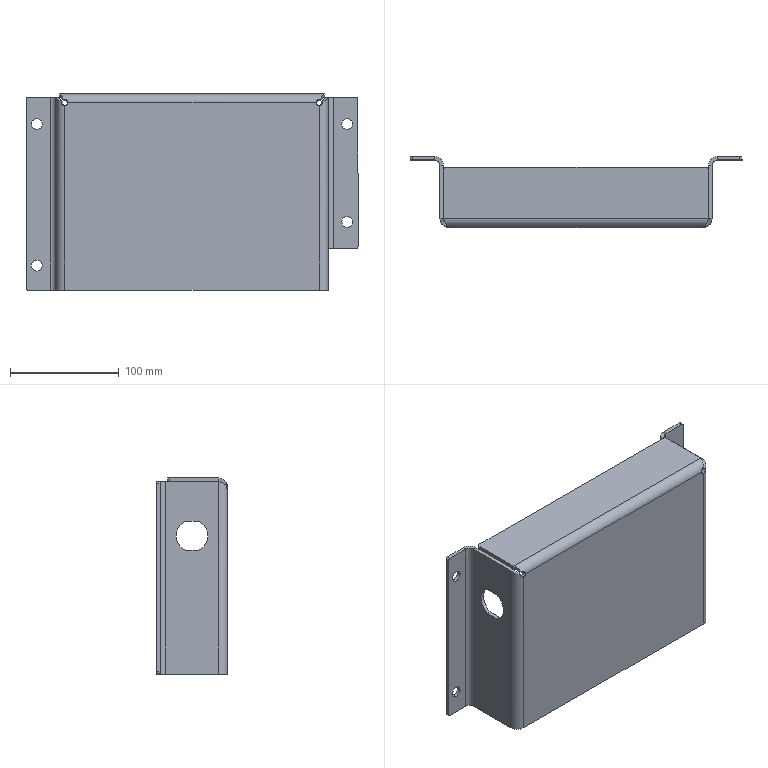Part | SolidWorks | features ICE 3, EdgeFlange 2, Fillet 1, FlatPattern 1, Fold 1, SMBaseFlange 1, SheetMetal 1, UnFold 1 | 1 solid | 80 faces | box 305 x 65 x 180.2 mm | volume 266620 mm3 | plane 38 | cylinder 34 | spline 8 | commonest cylinder face diameters 10 x13 4 x8 29.21 x6 16.4 x5 5 x2